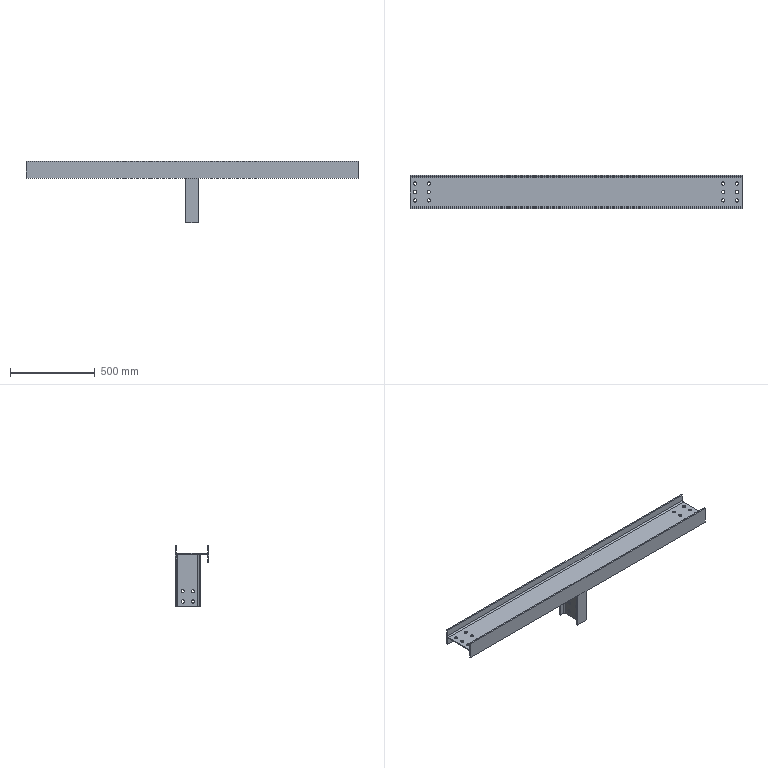Part | STEP file | 粉仓主梁14主体_Default<As Machined> | 2 solids | 71 faces | box 1955 x 200 x 360 mm | volume 5712085 mm3 | cylinder 40 | plane 31 | commonest cylinder face diameters 19 x32 16 x8